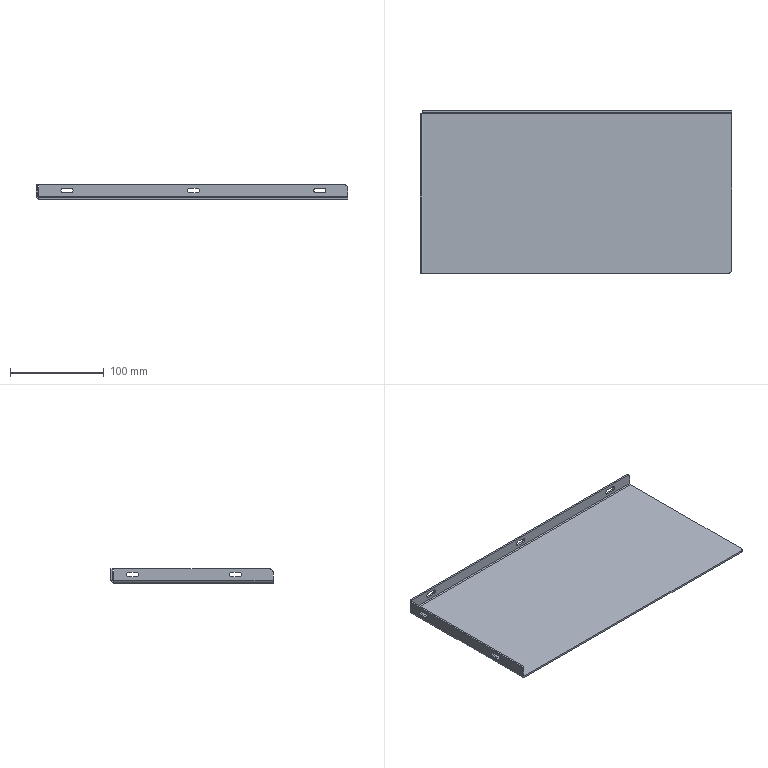Part | NX | features BREP 1 | 1 solid | 45 faces | box 333 x 173 x 15 mm | volume 126734 mm3 | plane 28 | cylinder 17 | commonest cylinder face diameters 5 x10 6 x5 2 x2
STEP:
#1=CARTESIAN_POINT('',(-168.,-85.,10.));
#2=VERTEX_POINT('',#1);
#3=CARTESIAN_POINT('',(-168.,-82.,13.));
#4=VERTEX_POINT('',#3);
#5=CARTESIAN_POINT('',(-168.,-82.,10.));
#6=DIRECTION('',(-1.,0.,0.));
#7=DIRECTION('',(0.,0.,-1.));
#8=AXIS2_PLACEMENT_3D('',#5,#6,#7);
#9=CIRCLE('',#8,3.);
#10=EDGE_CURVE('',#2,#4,#9,.T.);
#11=ORIENTED_EDGE('',*,*,#10,.F.);
#12=CARTESIAN_POINT('',(-166.,-85.,10.));
#13=VERTEX_POINT('',#12);
#14=CARTESIAN_POINT('',(-168.,-85.,10.));
#15=DIRECTION('',(-1.,0.,0.));
#16=VECTOR('',#15,1000.);
#17=LINE('',#14,#16);
#18=EDGE_CURVE('',#13,#2,#17,.T.);
#19=ORIENTED_EDGE('',*,*,#18,.F.);
#20=CARTESIAN_POINT('',(-166.,-82.,13.));
#21=VERTEX_POINT('',#20);
#22=CARTESIAN_POINT('',(-166.,-82.,10.));
#23=DIRECTION('',(1.,0.,0.));
#24=DIRECTION('',(0.,0.,-1.));
#25=AXIS2_PLACEMENT_3D('',#22,#23,#24);
#26=CIRCLE('',#25,3.);
#27=EDGE_CURVE('',#21,#13,#26,.T.);
#28=ORIENTED_EDGE('',*,*,#27,.F.);
#29=CARTESIAN_POINT('',(-168.,-82.,13.));
#30=DIRECTION('',(1.,0.,0.));
#31=VECTOR('',#30,1000.);
#32=LINE('',#29,#31);
#33=EDGE_CURVE('',#4,#21,#32,.T.);
#34=ORIENTED_EDGE('',*,*,#33,.F.);
#35=EDGE_LOOP('',(#11,#19,#28,#34));
#36=FACE_BOUND('',#35,.T.);
#37=CARTESIAN_POINT('',(-168.,-82.,10.));
#38=DIRECTION('',(1.,0.,0.));
#39=DIRECTION('',(0.,0.,-1.));
#40=AXIS2_PLACEMENT_3D('',#37,#38,#39);
#41=CYLINDRICAL_SURFACE('',#40,3.);
#42=ADVANCED_FACE('',(#36),#41,.T.);
#43=CARTESIAN_POINT('',(165.,-82.,-2.));
#44=VERTEX_POINT('',#43);
#45=CARTESIAN_POINT('',(162.,-85.,-2.));
#46=VERTEX_POINT('',#45);
#47=CARTESIAN_POINT('',(162.,-82.,-2.));
#48=DIRECTION('',(0.,0.,-1.));
#49=DIRECTION('',(-1.,0.,0.));
#50=AXIS2_PLACEMENT_3D('',#47,#48,#49);
#51=CIRCLE('',#50,3.);
#52=EDGE_CURVE('',#44,#46,#51,.T.);
#53=ORIENTED_EDGE('',*,*,#52,.F.);
#54=CARTESIAN_POINT('',(165.,-82.,0.));
#55=VERTEX_POINT('',#54);
#56=CARTESIAN_POINT('',(165.,-82.,-2.));
#57=DIRECTION('',(0.,0.,-1.));
#58=VECTOR('',#57,1000.);
#59=LINE('',#56,#58);
#60=EDGE_CURVE('',#55,#44,#59,.T.);
#61=ORIENTED_EDGE('',*,*,#60,.F.);
#62=CARTESIAN_POINT('',(162.,-85.,0.));
#63=VERTEX_POINT('',#62);
#64=CARTESIAN_POINT('',(162.,-82.,0.));
#65=DIRECTION('',(0.,0.,1.));
#66=DIRECTION('',(-1.,0.,0.));
#67=AXIS2_PLACEMENT_3D('',#64,#65,#66);
#68=CIRCLE('',#67,3.);
#69=EDGE_CURVE('',#63,#55,#68,.T.);
#70=ORIENTED_EDGE('',*,*,#69,.F.);
#71=CARTESIAN_POINT('',(162.,-85.,-2.));
#72=DIRECTION('',(0.,0.,1.));
#73=VECTOR('',#72,1000.);
#74=LINE('',#71,#73);
#75=EDGE_CURVE('',#46,#63,#74,.T.);
#76=ORIENTED_EDGE('',*,*,#75,.F.);
#77=EDGE_LOOP('',(#53,#61,#70,#76));
#78=FACE_BOUND('',#77,.T.);
#79=CARTESIAN_POINT('',(162.,-82.,-2.));
#80=DIRECTION('',(0.,0.,1.));
#81=DIRECTION('',(1.,0.,0.));
#82=AXIS2_PLACEMENT_3D('',#79,#80,#81);
#83=CYLINDRICAL_SURFACE('',#82,3.);
#84=ADVANCED_FACE('',(#78),#83,.T.);
#85=CARTESIAN_POINT('',(162.,88.,13.));
#86=VERTEX_POINT('',#85);
#87=CARTESIAN_POINT('',(165.,88.,10.));
#88=VERTEX_POINT('',#87);
#89=CARTESIAN_POINT('',(162.,88.,10.));
#90=DIRECTION('',(0.,1.,0.));
#91=DIRECTION('',(0.,0.,-1.));
#92=AXIS2_PLACEMENT_3D('',#89,#90,#91);
#93=CIRCLE('',#92,3.);
#94=EDGE_CURVE('',#86,#88,#93,.T.);
#95=ORIENTED_EDGE('',*,*,#94,.F.);
#96=CARTESIAN_POINT('',(162.,86.,13.));
#97=VERTEX_POINT('',#96);
#98=CARTESIAN_POINT('',(162.,88.,13.));
#99=DIRECTION('',(0.,1.,0.));
#100=VECTOR('',#99,1000.);
#101=LINE('',#98,#100);
#102=EDGE_CURVE('',#97,#86,#101,.T.);
#103=ORIENTED_EDGE('',*,*,#102,.F.);
#104=CARTESIAN_POINT('',(165.,86.,10.));
#105=VERTEX_POINT('',#104);
#106=CARTESIAN_POINT('',(162.,86.,10.));
#107=DIRECTION('',(0.,-1.,0.));
#108=DIRECTION('',(0.,0.,-1.));
#109=AXIS2_PLACEMENT_3D('',#106,#107,#108);
#110=CIRCLE('',#109,3.);
#111=EDGE_CURVE('',#105,#97,#110,.T.);
#112=ORIENTED_EDGE('',*,*,#111,.F.);
#113=CARTESIAN_POINT('',(165.,88.,10.));
#114=DIRECTION('',(0.,-1.,0.));
#115=VECTOR('',#114,1000.);
#116=LINE('',#113,#115);
#117=EDGE_CURVE('',#88,#105,#116,.T.);
#118=ORIENTED_EDGE('',*,*,#117,.F.);
#119=EDGE_LOOP('',(#95,#103,#112,#118));
#120=FACE_BOUND('',#119,.T.);
#121=CARTESIAN_POINT('',(162.,88.,10.));
#122=DIRECTION('',(0.,-1.,0.));
#123=DIRECTION('',(0.,0.,-1.));
#124=AXIS2_PLACEMENT_3D('',#121,#122,#123);
#125=CYLINDRICAL_SURFACE('',#124,3.);
#126=ADVANCED_FACE('',(#120),#125,.T.);
#127=CARTESIAN_POINT('',(-166.,-49.,4.5));
#128=VERTEX_POINT('',#127);
#129=CARTESIAN_POINT('',(-166.,-41.,4.5));
#130=VERTEX_POINT('',#129);
#131=CARTESIAN_POINT('',(-166.,-49.,4.5));
#132=DIRECTION('',(0.,1.,0.));
#133=VECTOR('',#132,1000.);
#134=LINE('',#131,#133);
#135=EDGE_CURVE('',#128,#130,#134,.T.);
#136=ORIENTED_EDGE('',*,*,#135,.T.);
#137=CARTESIAN_POINT('',(-168.,-41.,4.5));
#138=VERTEX_POINT('',#137);
#139=CARTESIAN_POINT('',(-168.,-41.,4.5));
#140=DIRECTION('',(1.,0.,0.));
#141=VECTOR('',#140,1000.);
#142=LINE('',#139,#141);
#143=EDGE_CURVE('',#138,#130,#142,.T.);
#144=ORIENTED_EDGE('',*,*,#143,.F.);
#145=CARTESIAN_POINT('',(-168.,-49.,4.5));
#146=VERTEX_POINT('',#145);
#147=CARTESIAN_POINT('',(-168.,-49.,4.5));
#148=DIRECTION('',(0.,1.,0.));
#149=VECTOR('',#148,1000.);
#150=LINE('',#147,#149);
#151=EDGE_CURVE('',#146,#138,#150,.T.);
#152=ORIENTED_EDGE('',*,*,#151,.F.);
#153=CARTESIAN_POINT('',(-168.,-49.,4.5));
#154=DIRECTION('',(1.,0.,0.));
#155=VECTOR('',#154,1000.);
#156=LINE('',#153,#155);
#157=EDGE_CURVE('',#146,#128,#156,.T.);
#158=ORIENTED_EDGE('',*,*,#157,.T.);
#159=EDGE_LOOP('',(#136,#144,#152,#158));
#160=FACE_BOUND('',#159,.T.);
#161=CARTESIAN_POINT('',(-168.,-49.,4.5));
#162=DIRECTION('',(0.,0.,-1.));
#163=DIRECTION('',(-1.,0.,0.));
#164=AXIS2_PLACEMENT_3D('',#161,#162,#163);
#165=PLANE('',#164);
#166=ADVANCED_FACE('',(#160),#165,.F.);
#167=CARTESIAN_POINT('',(-166.,-41.,9.5));
#168=VERTEX_POINT('',#167);
#169=CARTESIAN_POINT('',(-166.,-41.,7.));
#170=DIRECTION('',(1.,0.,0.));
#171=DIRECTION('',(0.,0.,-1.));
#172=AXIS2_PLACEMENT_3D('',#169,#170,#171);
#173=CIRCLE('',#172,2.5);
#174=EDGE_CURVE('',#130,#168,#173,.T.);
#175=ORIENTED_EDGE('',*,*,#174,.T.);
#176=CARTESIAN_POINT('',(-168.,-41.,9.5));
#177=VERTEX_POINT('',#176);
#178=CARTESIAN_POINT('',(-168.,-41.,9.5));
#179=DIRECTION('',(1.,0.,0.));
#180=VECTOR('',#179,1000.);
#181=LINE('',#178,#180);
#182=EDGE_CURVE('',#177,#168,#181,.T.);
#183=ORIENTED_EDGE('',*,*,#182,.F.);
#184=CARTESIAN_POINT('',(-168.,-41.,7.));
#185=DIRECTION('',(1.,0.,0.));
#186=DIRECTION('',(0.,0.,-1.));
#187=AXIS2_PLACEMENT_3D('',#184,#185,#186);
#188=CIRCLE('',#187,2.5);
#189=EDGE_CURVE('',#138,#177,#188,.T.);
#190=ORIENTED_EDGE('',*,*,#189,.F.);
#191=ORIENTED_EDGE('',*,*,#143,.T.);
#192=EDGE_LOOP('',(#175,#183,#190,#191));
#193=FACE_BOUND('',#192,.T.);
#194=CARTESIAN_POINT('',(-168.,-41.,7.));
#195=DIRECTION('',(1.,0.,0.));
#196=DIRECTION('',(0.,0.,-1.));
#197=AXIS2_PLACEMENT_3D('',#194,#195,#196);
#198=CYLINDRICAL_SURFACE('',#197,2.5);
#199=ADVANCED_FACE('',(#193),#198,.F.);
#200=CARTESIAN_POINT('',(-166.,-49.,9.5));
#201=VERTEX_POINT('',#200);
#202=CARTESIAN_POINT('',(-166.,-49.,9.5));
#203=DIRECTION('',(0.,-1.,0.));
#204=VECTOR('',#203,1000.);
#205=LINE('',#202,#204);
#206=EDGE_CURVE('',#168,#201,#205,.T.);
#207=ORIENTED_EDGE('',*,*,#206,.T.);
#208=CARTESIAN_POINT('',(-168.,-49.,9.5));
#209=VERTEX_POINT('',#208);
#210=CARTESIAN_POINT('',(-168.,-49.,9.5));
#211=DIRECTION('',(1.,0.,0.));
#212=VECTOR('',#211,1000.);
#213=LINE('',#210,#212);
#214=EDGE_CURVE('',#209,#201,#213,.T.);
#215=ORIENTED_EDGE('',*,*,#214,.F.);
#216=CARTESIAN_POINT('',(-168.,-49.,9.5));
#217=DIRECTION('',(0.,-1.,0.));
#218=VECTOR('',#217,1000.);
#219=LINE('',#216,#218);
#220=EDGE_CURVE('',#177,#209,#219,.T.);
#221=ORIENTED_EDGE('',*,*,#220,.F.);
#222=ORIENTED_EDGE('',*,*,#182,.T.);
#223=EDGE_LOOP('',(#207,#215,#221,#222));
#224=FACE_BOUND('',#223,.T.);
#225=CARTESIAN_POINT('',(-168.,-49.,9.5));
#226=DIRECTION('',(0.,0.,1.));
#227=DIRECTION('',(1.,0.,0.));
#228=AXIS2_PLACEMENT_3D('',#225,#226,#227);
#229=PLANE('',#228);
#230=ADVANCED_FACE('',(#224),#229,.F.);
#231=CARTESIAN_POINT('',(-166.,-49.,7.));
#232=DIRECTION('',(1.,0.,0.));
#233=DIRECTION('',(0.,0.,-1.));
#234=AXIS2_PLACEMENT_3D('',#231,#232,#233);
#235=CIRCLE('',#234,2.5);
#236=EDGE_CURVE('',#201,#128,#235,.T.);
#237=ORIENTED_EDGE('',*,*,#236,.T.);
#238=ORIENTED_EDGE('',*,*,#157,.F.);
#239=CARTESIAN_POINT('',(-168.,-49.,7.));
#240=DIRECTION('',(1.,0.,0.));
#241=DIRECTION('',(0.,0.,-1.));
#242=AXIS2_PLACEMENT_3D('',#239,#240,#241);
#243=CIRCLE('',#242,2.5);
#244=EDGE_CURVE('',#209,#146,#243,.T.);
#245=ORIENTED_EDGE('',*,*,#244,.F.);
#246=ORIENTED_EDGE('',*,*,#214,.T.);
#247=EDGE_LOOP('',(#237,#238,#245,#246));
#248=FACE_BOUND('',#247,.T.);
#249=CARTESIAN_POINT('',(-168.,-49.,7.));
#250=DIRECTION('',(1.,0.,0.));
#251=DIRECTION('',(0.,0.,-1.));
#252=AXIS2_PLACEMENT_3D('',#249,#250,#251);
#253=CYLINDRICAL_SURFACE('',#252,2.5);
#254=ADVANCED_FACE('',(#248),#253,.F.);
#255=CARTESIAN_POINT('',(-166.,61.,4.5));
#256=VERTEX_POINT('',#255);
#257=CARTESIAN_POINT('',(-166.,69.,4.5));
#258=VERTEX_POINT('',#257);
#259=CARTESIAN_POINT('',(-166.,61.,4.5));
#260=DIRECTION('',(0.,1.,0.));
#261=VECTOR('',#260,1000.);
#262=LINE('',#259,#261);
#263=EDGE_CURVE('',#256,#258,#262,.T.);
#264=ORIENTED_EDGE('',*,*,#263,.T.);
#265=CARTESIAN_POINT('',(-168.,69.,4.5));
#266=VERTEX_POINT('',#265);
#267=CARTESIAN_POINT('',(-168.,69.,4.5));
#268=DIRECTION('',(1.,0.,0.));
#269=VECTOR('',#268,1000.);
#270=LINE('',#267,#269);
#271=EDGE_CURVE('',#266,#258,#270,.T.);
#272=ORIENTED_EDGE('',*,*,#271,.F.);
#273=CARTESIAN_POINT('',(-168.,61.,4.5));
#274=VERTEX_POINT('',#273);
#275=CARTESIAN_POINT('',(-168.,61.,4.5));
#276=DIRECTION('',(0.,1.,0.));
#277=VECTOR('',#276,1000.);
#278=LINE('',#275,#277);
#279=EDGE_CURVE('',#274,#266,#278,.T.);
#280=ORIENTED_EDGE('',*,*,#279,.F.);
#281=CARTESIAN_POINT('',(-168.,61.,4.5));
#282=DIRECTION('',(1.,0.,0.));
#283=VECTOR('',#282,1000.);
#284=LINE('',#281,#283);
#285=EDGE_CURVE('',#274,#256,#284,.T.);
#286=ORIENTED_EDGE('',*,*,#285,.T.);
#287=EDGE_LOOP('',(#264,#272,#280,#286));
#288=FACE_BOUND('',#287,.T.);
#289=CARTESIAN_POINT('',(-168.,61.,4.5));
#290=DIRECTION('',(0.,0.,-1.));
#291=DIRECTION('',(-1.,0.,0.));
#292=AXIS2_PLACEMENT_3D('',#289,#290,#291);
#293=PLANE('',#292);
#294=ADVANCED_FACE('',(#288),#293,.F.);
#295=CARTESIAN_POINT('',(-166.,69.,9.5));
#296=VERTEX_POINT('',#295);
#297=CARTESIAN_POINT('',(-166.,69.,7.));
#298=DIRECTION('',(1.,0.,0.));
#299=DIRECTION('',(0.,0.,-1.));
#300=AXIS2_PLACEMENT_3D('',#297,#298,#299);
#301=CIRCLE('',#300,2.5);
#302=EDGE_CURVE('',#258,#296,#301,.T.);
#303=ORIENTED_EDGE('',*,*,#302,.T.);
#304=CARTESIAN_POINT('',(-168.,69.,9.5));
#305=VERTEX_POINT('',#304);
#306=CARTESIAN_POINT('',(-168.,69.,9.5));
#307=DIRECTION('',(1.,0.,0.));
#308=VECTOR('',#307,1000.);
#309=LINE('',#306,#308);
#310=EDGE_CURVE('',#305,#296,#309,.T.);
#311=ORIENTED_EDGE('',*,*,#310,.F.);
#312=CARTESIAN_POINT('',(-168.,69.,7.));
#313=DIRECTION('',(1.,0.,0.));
#314=DIRECTION('',(0.,0.,-1.));
#315=AXIS2_PLACEMENT_3D('',#312,#313,#314);
#316=CIRCLE('',#315,2.5);
#317=EDGE_CURVE('',#266,#305,#316,.T.);
#318=ORIENTED_EDGE('',*,*,#317,.F.);
#319=ORIENTED_EDGE('',*,*,#271,.T.);
#320=EDGE_LOOP('',(#303,#311,#318,#319));
#321=FACE_BOUND('',#320,.T.);
#322=CARTESIAN_POINT('',(-168.,69.,7.));
#323=DIRECTION('',(1.,0.,0.));
#324=DIRECTION('',(0.,0.,-1.));
#325=AXIS2_PLACEMENT_3D('',#322,#323,#324);
#326=CYLINDRICAL_SURFACE('',#325,2.5);
#327=ADVANCED_FACE('',(#321),#326,.F.);
#328=CARTESIAN_POINT('',(-166.,61.,9.5));
#329=VERTEX_POINT('',#328);
#330=CARTESIAN_POINT('',(-166.,61.,9.5));
#331=DIRECTION('',(0.,-1.,0.));
#332=VECTOR('',#331,1000.);
#333=LINE('',#330,#332);
#334=EDGE_CURVE('',#296,#329,#333,.T.);
#335=ORIENTED_EDGE('',*,*,#334,.T.);
#336=CARTESIAN_POINT('',(-168.,61.,9.5));
#337=VERTEX_POINT('',#336);
#338=CARTESIAN_POINT('',(-168.,61.,9.5));
#339=DIRECTION('',(1.,0.,0.));
#340=VECTOR('',#339,1000.);
#341=LINE('',#338,#340);
#342=EDGE_CURVE('',#337,#329,#341,.T.);
#343=ORIENTED_EDGE('',*,*,#342,.F.);
#344=CARTESIAN_POINT('',(-168.,61.,9.5));
#345=DIRECTION('',(0.,-1.,0.));
#346=VECTOR('',#345,1000.);
#347=LINE('',#344,#346);
#348=EDGE_CURVE('',#305,#337,#347,.T.);
#349=ORIENTED_EDGE('',*,*,#348,.F.);
#350=ORIENTED_EDGE('',*,*,#310,.T.);
#351=EDGE_LOOP('',(#335,#343,#349,#350));
#352=FACE_BOUND('',#351,.T.);
#353=CARTESIAN_POINT('',(-168.,61.,9.5));
#354=DIRECTION('',(0.,0.,1.));
#355=DIRECTION('',(1.,0.,0.));
#356=AXIS2_PLACEMENT_3D('',#353,#354,#355);
#357=PLANE('',#356);
#358=ADVANCED_FACE('',(#352),#357,.F.);
#359=CARTESIAN_POINT('',(-166.,61.,7.));
#360=DIRECTION('',(1.,0.,0.));
#361=DIRECTION('',(0.,0.,-1.));
#362=AXIS2_PLACEMENT_3D('',#359,#360,#361);
#363=CIRCLE('',#362,2.5);
#364=EDGE_CURVE('',#329,#256,#363,.T.);
#365=ORIENTED_EDGE('',*,*,#364,.T.);
#366=ORIENTED_EDGE('',*,*,#285,.F.);
#367=CARTESIAN_POINT('',(-168.,61.,7.));
#368=DIRECTION('',(1.,0.,0.));
#369=DIRECTION('',(0.,0.,-1.));
#370=AXIS2_PLACEMENT_3D('',#367,#368,#369);
#371=CIRCLE('',#370,2.5);
#372=EDGE_CURVE('',#337,#274,#371,.T.);
#373=ORIENTED_EDGE('',*,*,#372,.F.);
#374=ORIENTED_EDGE('',*,*,#342,.T.);
#375=EDGE_LOOP('',(#365,#366,#373,#374));
#376=FACE_BOUND('',#375,.T.);
#377=CARTESIAN_POINT('',(-168.,61.,7.));
#378=DIRECTION('',(1.,0.,0.));
#379=DIRECTION('',(0.,0.,-1.));
#380=AXIS2_PLACEMENT_3D('',#377,#378,#379);
#381=CYLINDRICAL_SURFACE('',#380,2.5);
#382=ADVANCED_FACE('',(#376),#381,.F.);
#383=CARTESIAN_POINT('',(4.,86.,9.5));
#384=VERTEX_POINT('',#383);
#385=CARTESIAN_POINT('',(-4.,86.,9.5));
#386=VERTEX_POINT('',#385);
#387=CARTESIAN_POINT('',(4.,86.,9.5));
#388=DIRECTION('',(-1.,0.,0.));
#389=VECTOR('',#388,1000.);
#390=LINE('',#387,#389);
#391=EDGE_CURVE('',#384,#386,#390,.T.);
#392=ORIENTED_EDGE('',*,*,#391,.T.);
#393=CARTESIAN_POINT('',(-4.,88.,9.5));
#394=VERTEX_POINT('',#393);
#395=CARTESIAN_POINT('',(-4.,88.,9.5));
#396=DIRECTION('',(0.,-1.,0.));
#397=VECTOR('',#396,1000.);
#398=LINE('',#395,#397);
#399=EDGE_CURVE('',#394,#386,#398,.T.);
#400=ORIENTED_EDGE('',*,*,#399,.F.);
#401=CARTESIAN_POINT('',(4.,88.,9.5));
#402=VERTEX_POINT('',#401);
#403=CARTESIAN_POINT('',(4.,88.,9.5));
#404=DIRECTION('',(-1.,0.,0.));
#405=VECTOR('',#404,1000.);
#406=LINE('',#403,#405);
#407=EDGE_CURVE('',#402,#394,#406,.T.);
#408=ORIENTED_EDGE('',*,*,#407,.F.);
#409=CARTESIAN_POINT('',(4.,88.,9.5));
#410=DIRECTION('',(0.,-1.,0.));
#411=VECTOR('',#410,1000.);
#412=LINE('',#409,#411);
#413=EDGE_CURVE('',#402,#384,#412,.T.);
#414=ORIENTED_EDGE('',*,*,#413,.T.);
#415=EDGE_LOOP('',(#392,#400,#408,#414));
#416=FACE_BOUND('',#415,.T.);
#417=CARTESIAN_POINT('',(4.,88.,9.5));
#418=DIRECTION('',(0.,0.,1.));
#419=DIRECTION('',(0.,-1.,0.));
#420=AXIS2_PLACEMENT_3D('',#417,#418,#419);
#421=PLANE('',#420);
#422=ADVANCED_FACE('',(#416),#421,.F.);
#423=CARTESIAN_POINT('',(-4.,86.,4.5));
#424=VERTEX_POINT('',#423);
#425=CARTESIAN_POINT('',(-4.,86.,7.));
#426=DIRECTION('',(0.,-1.,0.));
#427=DIRECTION('',(0.,0.,-1.));
#428=AXIS2_PLACEMENT_3D('',#425,#426,#427);
#429=CIRCLE('',#428,2.5);
#430=EDGE_CURVE('',#386,#424,#429,.T.);
#431=ORIENTED_EDGE('',*,*,#430,.T.);
#432=CARTESIAN_POINT('',(-4.,88.,4.5));
#433=VERTEX_POINT('',#432);
#434=CARTESIAN_POINT('',(-4.,88.,4.5));
#435=DIRECTION('',(0.,-1.,0.));
#436=VECTOR('',#435,1000.);
#437=LINE('',#434,#436);
#438=EDGE_CURVE('',#433,#424,#437,.T.);
#439=ORIENTED_EDGE('',*,*,#438,.F.);
#440=CARTESIAN_POINT('',(-4.,88.,7.));
#441=DIRECTION('',(0.,-1.,0.));
#442=DIRECTION('',(0.,0.,-1.));
#443=AXIS2_PLACEMENT_3D('',#440,#441,#442);
#444=CIRCLE('',#443,2.5);
#445=EDGE_CURVE('',#394,#433,#444,.T.);
#446=ORIENTED_EDGE('',*,*,#445,.F.);
#447=ORIENTED_EDGE('',*,*,#399,.T.);
#448=EDGE_LOOP('',(#431,#439,#446,#447));
#449=FACE_BOUND('',#448,.T.);
#450=CARTESIAN_POINT('',(-4.,88.,7.));
#451=DIRECTION('',(0.,-1.,0.));
#452=DIRECTION('',(0.,0.,-1.));
#453=AXIS2_PLACEMENT_3D('',#450,#451,#452);
#454=CYLINDRICAL_SURFACE('',#453,2.5);
#455=ADVANCED_FACE('',(#449),#454,.F.);
#456=CARTESIAN_POINT('',(4.,86.,4.5));
#457=VERTEX_POINT('',#456);
#458=CARTESIAN_POINT('',(4.,86.,4.5));
#459=DIRECTION('',(1.,0.,0.));
#460=VECTOR('',#459,1000.);
#461=LINE('',#458,#460);
#462=EDGE_CURVE('',#424,#457,#461,.T.);
#463=ORIENTED_EDGE('',*,*,#462,.T.);
#464=CARTESIAN_POINT('',(4.,88.,4.5));
#465=VERTEX_POINT('',#464);
#466=CARTESIAN_POINT('',(4.,88.,4.5));
#467=DIRECTION('',(0.,-1.,0.));
#468=VECTOR('',#467,1000.);
#469=LINE('',#466,#468);
#470=EDGE_CURVE('',#465,#457,#469,.T.);
#471=ORIENTED_EDGE('',*,*,#470,.F.);
#472=CARTESIAN_POINT('',(4.,88.,4.5));
#473=DIRECTION('',(1.,0.,0.));
#474=VECTOR('',#473,1000.);
#475=LINE('',#472,#474);
#476=EDGE_CURVE('',#433,#465,#475,.T.);
#477=ORIENTED_EDGE('',*,*,#476,.F.);
#478=ORIENTED_EDGE('',*,*,#438,.T.);
#479=EDGE_LOOP('',(#463,#471,#477,#478));
#480=FACE_BOUND('',#479,.T.);
#481=CARTESIAN_POINT('',(4.,88.,4.5));
#482=DIRECTION('',(0.,0.,-1.));
#483=DIRECTION('',(0.,1.,0.));
#484=AXIS2_PLACEMENT_3D('',#481,#482,#483);
#485=PLANE('',#484);
#486=ADVANCED_FACE('',(#480),#485,.F.);
#487=CARTESIAN_POINT('',(4.,86.,7.));
#488=DIRECTION('',(0.,-1.,0.));
#489=DIRECTION('',(0.,0.,-1.));
#490=AXIS2_PLACEMENT_3D('',#487,#488,#489);
#491=CIRCLE('',#490,2.5);
#492=EDGE_CURVE('',#457,#384,#491,.T.);
#493=ORIENTED_EDGE('',*,*,#492,.T.);
#494=ORIENTED_EDGE('',*,*,#413,.F.);
#495=CARTESIAN_POINT('',(4.,88.,7.));
#496=DIRECTION('',(0.,-1.,0.));
#497=DIRECTION('',(0.,0.,-1.));
#498=AXIS2_PLACEMENT_3D('',#495,#496,#497);
#499=CIRCLE('',#498,2.5);
#500=EDGE_CURVE('',#465,#402,#499,.T.);
#501=ORIENTED_EDGE('',*,*,#500,.F.);
#502=ORIENTED_EDGE('',*,*,#470,.T.);
#503=EDGE_LOOP('',(#493,#494,#501,#502));
#504=FACE_BOUND('',#503,.T.);
#505=CARTESIAN_POINT('',(4.,88.,7.));
#506=DIRECTION('',(0.,-1.,0.));
#507=DIRECTION('',(0.,0.,-1.));
#508=AXIS2_PLACEMENT_3D('',#505,#506,#507);
#509=CYLINDRICAL_SURFACE('',#508,2.5);
#510=ADVANCED_FACE('',(#504),#509,.F.);
#511=CARTESIAN_POINT('',(-131.,86.,9.5));
#512=VERTEX_POINT('',#511);
#513=CARTESIAN_POINT('',(-139.,86.,9.5));
#514=VERTEX_POINT('',#513);
#515=CARTESIAN_POINT('',(-131.,86.,9.5));
#516=DIRECTION('',(-1.,0.,0.));
#517=VECTOR('',#516,1000.);
#518=LINE('',#515,#517);
#519=EDGE_CURVE('',#512,#514,#518,.T.);
#520=ORIENTED_EDGE('',*,*,#519,.T.);
#521=CARTESIAN_POINT('',(-139.,88.,9.5));
#522=VERTEX_POINT('',#521);
#523=CARTESIAN_POINT('',(-139.,88.,9.5));
#524=DIRECTION('',(0.,-1.,0.));
#525=VECTOR('',#524,1000.);
#526=LINE('',#523,#525);
#527=EDGE_CURVE('',#522,#514,#526,.T.);
#528=ORIENTED_EDGE('',*,*,#527,.F.);
#529=CARTESIAN_POINT('',(-131.,88.,9.5));
#530=VERTEX_POINT('',#529);
#531=CARTESIAN_POINT('',(-131.,88.,9.5));
#532=DIRECTION('',(-1.,0.,0.));
#533=VECTOR('',#532,1000.);
#534=LINE('',#531,#533);
#535=EDGE_CURVE('',#530,#522,#534,.T.);
#536=ORIENTED_EDGE('',*,*,#535,.F.);
#537=CARTESIAN_POINT('',(-131.,88.,9.5));
#538=DIRECTION('',(0.,-1.,0.));
#539=VECTOR('',#538,1000.);
#540=LINE('',#537,#539);
#541=EDGE_CURVE('',#530,#512,#540,.T.);
#542=ORIENTED_EDGE('',*,*,#541,.T.);
#543=EDGE_LOOP('',(#520,#528,#536,#542));
#544=FACE_BOUND('',#543,.T.);
#545=CARTESIAN_POINT('',(-131.,88.,9.5));
#546=DIRECTION('',(0.,0.,1.));
#547=DIRECTION('',(0.,-1.,0.));
#548=AXIS2_PLACEMENT_3D('',#545,#546,#547);
#549=PLANE('',#548);
#550=ADVANCED_FACE('',(#544),#549,.F.);
#551=CARTESIAN_POINT('',(-139.,86.,4.5));
#552=VERTEX_POINT('',#551);
#553=CARTESIAN_POINT('',(-139.,86.,7.));
#554=DIRECTION('',(0.,-1.,0.));
#555=DIRECTION('',(0.,0.,-1.));
#556=AXIS2_PLACEMENT_3D('',#553,#554,#555);
#557=CIRCLE('',#556,2.5);
#558=EDGE_CURVE('',#514,#552,#557,.T.);
#559=ORIENTED_EDGE('',*,*,#558,.T.);
#560=CARTESIAN_POINT('',(-139.,88.,4.5));
#561=VERTEX_POINT('',#560);
#562=CARTESIAN_POINT('',(-139.,88.,4.5));
#563=DIRECTION('',(0.,-1.,0.));
#564=VECTOR('',#563,1000.);
#565=LINE('',#562,#564);
#566=EDGE_CURVE('',#561,#552,#565,.T.);
#567=ORIENTED_EDGE('',*,*,#566,.F.);
#568=CARTESIAN_POINT('',(-139.,88.,7.));
#569=DIRECTION('',(0.,-1.,0.));
#570=DIRECTION('',(0.,0.,-1.));
#571=AXIS2_PLACEMENT_3D('',#568,#569,#570);
#572=CIRCLE('',#571,2.5);
#573=EDGE_CURVE('',#522,#561,#572,.T.);
#574=ORIENTED_EDGE('',*,*,#573,.F.);
#575=ORIENTED_EDGE('',*,*,#527,.T.);
#576=EDGE_LOOP('',(#559,#567,#574,#575));
#577=FACE_BOUND('',#576,.T.);
#578=CARTESIAN_POINT('',(-139.,88.,7.));
#579=DIRECTION('',(0.,-1.,0.));
#580=DIRECTION('',(0.,0.,-1.));
#581=AXIS2_PLACEMENT_3D('',#578,#579,#580);
#582=CYLINDRICAL_SURFACE('',#581,2.5);
#583=ADVANCED_FACE('',(#577),#582,.F.);
#584=CARTESIAN_POINT('',(-131.,86.,4.5));
#585=VERTEX_POINT('',#584);
#586=CARTESIAN_POINT('',(-131.,86.,4.5));
#587=DIRECTION('',(1.,0.,0.));
#588=VECTOR('',#587,1000.);
#589=LINE('',#586,#588);
#590=EDGE_CURVE('',#552,#585,#589,.T.);
#591=ORIENTED_EDGE('',*,*,#590,.T.);
#592=CARTESIAN_POINT('',(-131.,88.,4.5));
#593=VERTEX_POINT('',#592);
#594=CARTESIAN_POINT('',(-131.,88.,4.5));
#595=DIRECTION('',(0.,-1.,0.));
#596=VECTOR('',#595,1000.);
#597=LINE('',#594,#596);
#598=EDGE_CURVE('',#593,#585,#597,.T.);
#599=ORIENTED_EDGE('',*,*,#598,.F.);
#600=CARTESIAN_POINT('',(-131.,88.,4.5));
#601=DIRECTION('',(1.,0.,0.));
#602=VECTOR('',#601,1000.);
#603=LINE('',#600,#602);
#604=EDGE_CURVE('',#561,#593,#603,.T.);
#605=ORIENTED_EDGE('',*,*,#604,.F.);
#606=ORIENTED_EDGE('',*,*,#566,.T.);
#607=EDGE_LOOP('',(#591,#599,#605,#606));
#608=FACE_BOUND('',#607,.T.);
#609=CARTESIAN_POINT('',(-131.,88.,4.5));
#610=DIRECTION('',(0.,0.,-1.));
#611=DIRECTION('',(0.,1.,0.));
#612=AXIS2_PLACEMENT_3D('',#609,#610,#611);
#613=PLANE('',#612);
#614=ADVANCED_FACE('',(#608),#613,.F.);
#615=CARTESIAN_POINT('',(-131.,86.,7.));
#616=DIRECTION('',(0.,-1.,0.));
#617=DIRECTION('',(0.,0.,-1.));
#618=AXIS2_PLACEMENT_3D('',#615,#616,#617);
#619=CIRCLE('',#618,2.5);
#620=EDGE_CURVE('',#585,#512,#619,.T.);
#621=ORIENTED_EDGE('',*,*,#620,.T.);
#622=ORIENTED_EDGE('',*,*,#541,.F.);
#623=CARTESIAN_POINT('',(-131.,88.,7.));
#624=DIRECTION('',(0.,-1.,0.));
#625=DIRECTION('',(0.,0.,-1.));
#626=AXIS2_PLACEMENT_3D('',#623,#624,#625);
#627=CIRCLE('',#626,2.5);
#628=EDGE_CURVE('',#593,#530,#627,.T.);
#629=ORIENTED_EDGE('',*,*,#628,.F.);
#630=ORIENTED_EDGE('',*,*,#598,.T.);
#631=EDGE_LOOP('',(#621,#622,#629,#630));
#632=FACE_BOUND('',#631,.T.);
#633=CARTESIAN_POINT('',(-131.,88.,7.));
#634=DIRECTION('',(0.,-1.,0.));
#635=DIRECTION('',(0.,0.,-1.));
#636=AXIS2_PLACEMENT_3D('',#633,#634,#635);
#637=CYLINDRICAL_SURFACE('',#636,2.5);
#638=ADVANCED_FACE('',(#632),#637,.F.);
#639=CARTESIAN_POINT('',(139.,86.,9.5));
#640=VERTEX_POINT('',#639);
#641=CARTESIAN_POINT('',(131.,86.,9.5));
#642=VERTEX_POINT('',#641);
#643=CARTESIAN_POINT('',(139.,86.,9.5));
#644=DIRECTION('',(-1.,0.,0.));
#645=VECTOR('',#644,1000.);
#646=LINE('',#643,#645);
#647=EDGE_CURVE('',#640,#642,#646,.T.);
#648=ORIENTED_EDGE('',*,*,#647,.T.);
#649=CARTESIAN_POINT('',(131.,88.,9.5));
#650=VERTEX_POINT('',#649);
#651=CARTESIAN_POINT('',(131.,88.,9.5));
#652=DIRECTION('',(0.,-1.,0.));
#653=VECTOR('',#652,1000.);
#654=LINE('',#651,#653);
#655=EDGE_CURVE('',#650,#642,#654,.T.);
#656=ORIENTED_EDGE('',*,*,#655,.F.);
#657=CARTESIAN_POINT('',(139.,88.,9.5));
#658=VERTEX_POINT('',#657);
#659=CARTESIAN_POINT('',(139.,88.,9.5));
#660=DIRECTION('',(-1.,0.,0.));
#661=VECTOR('',#660,1000.);
#662=LINE('',#659,#661);
#663=EDGE_CURVE('',#658,#650,#662,.T.);
#664=ORIENTED_EDGE('',*,*,#663,.F.);
#665=CARTESIAN_POINT('',(139.,88.,9.5));
#666=DIRECTION('',(0.,-1.,0.));
#667=VECTOR('',#666,1000.);
#668=LINE('',#665,#667);
#669=EDGE_CURVE('',#658,#640,#668,.T.);
#670=ORIENTED_EDGE('',*,*,#669,.T.);
#671=EDGE_LOOP('',(#648,#656,#664,#670));
#672=FACE_BOUND('',#671,.T.);
#673=CARTESIAN_POINT('',(139.,88.,9.5));
#674=DIRECTION('',(0.,0.,1.));
#675=DIRECTION('',(0.,-1.,0.));
#676=AXIS2_PLACEMENT_3D('',#673,#674,#675);
#677=PLANE('',#676);
#678=ADVANCED_FACE('',(#672),#677,.F.);
#679=CARTESIAN_POINT('',(131.,86.,4.5));
#680=VERTEX_POINT('',#679);
#681=CARTESIAN_POINT('',(131.,86.,7.));
#682=DIRECTION('',(0.,-1.,0.));
#683=DIRECTION('',(0.,0.,-1.));
#684=AXIS2_PLACEMENT_3D('',#681,#682,#683);
#685=CIRCLE('',#684,2.5);
#686=EDGE_CURVE('',#642,#680,#685,.T.);
#687=ORIENTED_EDGE('',*,*,#686,.T.);
#688=CARTESIAN_POINT('',(131.,88.,4.5));
#689=VERTEX_POINT('',#688);
#690=CARTESIAN_POINT('',(131.,88.,4.5));
#691=DIRECTION('',(0.,-1.,0.));
#692=VECTOR('',#691,1000.);
#693=LINE('',#690,#692);
#694=EDGE_CURVE('',#689,#680,#693,.T.);
#695=ORIENTED_EDGE('',*,*,#694,.F.);
#696=CARTESIAN_POINT('',(131.,88.,7.));
#697=DIRECTION('',(0.,-1.,0.));
#698=DIRECTION('',(0.,0.,-1.));
#699=AXIS2_PLACEMENT_3D('',#696,#697,#698);
#700=CIRCLE('',#699,2.5);
#701=EDGE_CURVE('',#650,#689,#700,.T.);
#702=ORIENTED_EDGE('',*,*,#701,.F.);
#703=ORIENTED_EDGE('',*,*,#655,.T.);
#704=EDGE_LOOP('',(#687,#695,#702,#703));
#705=FACE_BOUND('',#704,.T.);
#706=CARTESIAN_POINT('',(131.,88.,7.));
#707=DIRECTION('',(0.,-1.,0.));
#708=DIRECTION('',(0.,0.,-1.));
#709=AXIS2_PLACEMENT_3D('',#706,#707,#708);
#710=CYLINDRICAL_SURFACE('',#709,2.5);
#711=ADVANCED_FACE('',(#705),#710,.F.);
#712=CARTESIAN_POINT('',(139.,86.,4.5));
#713=VERTEX_POINT('',#712);
#714=CARTESIAN_POINT('',(139.,86.,4.5));
#715=DIRECTION('',(1.,0.,0.));
#716=VECTOR('',#715,1000.);
#717=LINE('',#714,#716);
#718=EDGE_CURVE('',#680,#713,#717,.T.);
#719=ORIENTED_EDGE('',*,*,#718,.T.);
#720=CARTESIAN_POINT('',(139.,88.,4.5));
#721=VERTEX_POINT('',#720);
#722=CARTESIAN_POINT('',(139.,88.,4.5));
#723=DIRECTION('',(0.,-1.,0.));
#724=VECTOR('',#723,1000.);
#725=LINE('',#722,#724);
#726=EDGE_CURVE('',#721,#713,#725,.T.);
#727=ORIENTED_EDGE('',*,*,#726,.F.);
#728=CARTESIAN_POINT('',(139.,88.,4.5));
#729=DIRECTION('',(1.,0.,0.));
#730=VECTOR('',#729,1000.);
#731=LINE('',#728,#730);
#732=EDGE_CURVE('',#689,#721,#731,.T.);
#733=ORIENTED_EDGE('',*,*,#732,.F.);
#734=ORIENTED_EDGE('',*,*,#694,.T.);
#735=EDGE_LOOP('',(#719,#727,#733,#734));
#736=FACE_BOUND('',#735,.T.);
#737=CARTESIAN_POINT('',(139.,88.,4.5));
#738=DIRECTION('',(0.,0.,-1.));
#739=DIRECTION('',(0.,1.,0.));
#740=AXIS2_PLACEMENT_3D('',#737,#738,#739);
#741=PLANE('',#740);
#742=ADVANCED_FACE('',(#736),#741,.F.);
#743=CARTESIAN_POINT('',(139.,86.,7.));
#744=DIRECTION('',(0.,-1.,0.));
#745=DIRECTION('',(0.,0.,-1.));
#746=AXIS2_PLACEMENT_3D('',#743,#744,#745);
#747=CIRCLE('',#746,2.5);
#748=EDGE_CURVE('',#713,#640,#747,.T.);
#749=ORIENTED_EDGE('',*,*,#748,.T.);
#750=ORIENTED_EDGE('',*,*,#669,.F.);
#751=CARTESIAN_POINT('',(139.,88.,7.));
#752=DIRECTION('',(0.,-1.,0.));
#753=DIRECTION('',(0.,0.,-1.));
#754=AXIS2_PLACEMENT_3D('',#751,#752,#753);
#755=CIRCLE('',#754,2.5);
#756=EDGE_CURVE('',#721,#658,#755,.T.);
#757=ORIENTED_EDGE('',*,*,#756,.F.);
#758=ORIENTED_EDGE('',*,*,#726,.T.);
#759=EDGE_LOOP('',(#749,#750,#757,#758));
#760=FACE_BOUND('',#759,.T.);
#761=CARTESIAN_POINT('',(139.,88.,7.));
#762=DIRECTION('',(0.,-1.,0.));
#763=DIRECTION('',(0.,0.,-1.));
#764=AXIS2_PLACEMENT_3D('',#761,#762,#763);
#765=CYLINDRICAL_SURFACE('',#764,2.5);
#766=ADVANCED_FACE('',(#760),#765,.F.);
#767=CARTESIAN_POINT('',(-168.,85.,13.));
#768=VERTEX_POINT('',#767);
#769=CARTESIAN_POINT('',(-168.,0.,13.));
#770=DIRECTION('',(0.,1.,0.));
#771=VECTOR('',#770,1000.);
#772=LINE('',#769,#771);
#773=EDGE_CURVE('',#4,#768,#772,.T.);
#774=ORIENTED_EDGE('',*,*,#773,.F.);
#775=ORIENTED_EDGE('',*,*,#33,.T.);
#776=CARTESIAN_POINT('',(-166.,85.,13.));
#777=VERTEX_POINT('',#776);
#778=CARTESIAN_POINT('',(-166.,85.,13.));
#779=DIRECTION('',(0.,1.,0.));
#780=VECTOR('',#779,1000.);
#781=LINE('',#778,#780);
#782=EDGE_CURVE('',#21,#777,#781,.T.);
#783=ORIENTED_EDGE('',*,*,#782,.T.);
#784=CARTESIAN_POINT('',(-168.,85.,13.));
#785=DIRECTION('',(1.,0.,0.));
#786=VECTOR('',#785,1000.);
#787=LINE('',#784,#786);
#788=EDGE_CURVE('',#768,#777,#787,.T.);
#789=ORIENTED_EDGE('',*,*,#788,.F.);
#790=EDGE_LOOP('',(#774,#775,#783,#789));
#791=FACE_BOUND('',#790,.T.);
#792=CARTESIAN_POINT('',(-168.,85.,13.));
#793=DIRECTION('',(0.,0.,-1.));
#794=DIRECTION('',(-1.,0.,0.));
#795=AXIS2_PLACEMENT_3D('',#792,#793,#794);
#796=PLANE('',#795);
#797=ADVANCED_FACE('',(#791),#796,.F.);
#798=ORIENTED_EDGE('',*,*,#782,.F.);
#799=ORIENTED_EDGE('',*,*,#27,.T.);
#800=CARTESIAN_POINT('',(-166.,-85.,1.));
#801=VERTEX_POINT('',#800);
#802=CARTESIAN_POINT('',(-166.,-85.,13.));
#803=DIRECTION('',(0.,0.,1.));
#804=VECTOR('',#803,1000.);
#805=LINE('',#802,#804);
#806=EDGE_CURVE('',#801,#13,#805,.T.);
#807=ORIENTED_EDGE('',*,*,#806,.F.);
#808=CARTESIAN_POINT('',(-166.,85.,1.));
#809=VERTEX_POINT('',#808);
#810=CARTESIAN_POINT('',(-166.,85.,1.));
#811=DIRECTION('',(0.,-1.,0.));
#812=VECTOR('',#811,1000.);
#813=LINE('',#810,#812);
#814=EDGE_CURVE('',#809,#801,#813,.T.);
#815=ORIENTED_EDGE('',*,*,#814,.F.);
#816=CARTESIAN_POINT('',(-166.,85.,0.));
#817=DIRECTION('',(0.,0.,-1.));
#818=VECTOR('',#817,1000.);
#819=LINE('',#816,#818);
#820=EDGE_CURVE('',#777,#809,#819,.T.);
#821=ORIENTED_EDGE('',*,*,#820,.F.);
#822=EDGE_LOOP('',(#798,#799,#807,#815,#821));
#823=FACE_BOUND('',#822,.T.);
#824=ORIENTED_EDGE('',*,*,#364,.F.);
#825=ORIENTED_EDGE('',*,*,#334,.F.);
#826=ORIENTED_EDGE('',*,*,#302,.F.);
#827=ORIENTED_EDGE('',*,*,#263,.F.);
#828=EDGE_LOOP('',(#824,#825,#826,#827));
#829=FACE_BOUND('',#828,.T.);
#830=ORIENTED_EDGE('',*,*,#236,.F.);
#831=ORIENTED_EDGE('',*,*,#206,.F.);
#832=ORIENTED_EDGE('',*,*,#174,.F.);
#833=ORIENTED_EDGE('',*,*,#135,.F.);
#834=EDGE_LOOP('',(#830,#831,#832,#833));
#835=FACE_BOUND('',#834,.T.);
#836=CARTESIAN_POINT('',(-166.,0.,0.));
#837=DIRECTION('',(1.,0.,0.));
#838=DIRECTION('',(0.,0.,-1.));
#839=AXIS2_PLACEMENT_3D('',#836,#837,#838);
#840=PLANE('',#839);
#841=ADVANCED_FACE('',(#823,#829,#835),#840,.T.);
#842=CARTESIAN_POINT('',(-168.,-85.,1.));
#843=VERTEX_POINT('',#842);
#844=CARTESIAN_POINT('',(-168.,-85.,0.));
#845=DIRECTION('',(0.,0.,1.));
#846=VECTOR('',#845,1000.);
#847=LINE('',#844,#846);
#848=EDGE_CURVE('',#843,#2,#847,.T.);
#849=ORIENTED_EDGE('',*,*,#848,.T.);
#850=ORIENTED_EDGE('',*,*,#10,.T.);
#851=ORIENTED_EDGE('',*,*,#773,.T.);
#852=CARTESIAN_POINT('',(-168.,85.,1.));
#853=VERTEX_POINT('',#852);
#854=CARTESIAN_POINT('',(-168.,85.,0.));
#855=DIRECTION('',(0.,0.,-1.));
#856=VECTOR('',#855,1000.);
#857=LINE('',#854,#856);
#858=EDGE_CURVE('',#768,#853,#857,.T.);
#859=ORIENTED_EDGE('',*,*,#858,.T.);
#860=CARTESIAN_POINT('',(-168.,85.,1.));
#861=DIRECTION('',(0.,1.,0.));
#862=VECTOR('',#861,1000.);
#863=LINE('',#860,#862);
#864=EDGE_CURVE('',#843,#853,#863,.T.);
#865=ORIENTED_EDGE('',*,*,#864,.F.);
#866=EDGE_LOOP('',(#849,#850,#851,#859,#865));
#867=FACE_BOUND('',#866,.T.);
#868=ORIENTED_EDGE('',*,*,#348,.T.);
#869=ORIENTED_EDGE('',*,*,#372,.T.);
#870=ORIENTED_EDGE('',*,*,#279,.T.);
#871=ORIENTED_EDGE('',*,*,#317,.T.);
#872=EDGE_LOOP('',(#868,#869,#870,#871));
#873=FACE_BOUND('',#872,.T.);
#874=ORIENTED_EDGE('',*,*,#220,.T.);
#875=ORIENTED_EDGE('',*,*,#244,.T.);
#876=ORIENTED_EDGE('',*,*,#151,.T.);
#877=ORIENTED_EDGE('',*,*,#189,.T.);
#878=EDGE_LOOP('',(#874,#875,#876,#877));
#879=FACE_BOUND('',#878,.T.);
#880=CARTESIAN_POINT('',(-168.,0.,0.));
#881=DIRECTION('',(1.,0.,0.));
#882=DIRECTION('',(0.,0.,-1.));
#883=AXIS2_PLACEMENT_3D('',#880,#881,#882);
#884=PLANE('',#883);
#885=ADVANCED_FACE('',(#867,#873,#879),#884,.F.);
#886=CARTESIAN_POINT('',(-168.,85.,1.));
#887=DIRECTION('',(-1.,0.,0.));
#888=VECTOR('',#887,1000.);
#889=LINE('',#886,#888);
#890=EDGE_CURVE('',#809,#853,#889,.T.);
#891=ORIENTED_EDGE('',*,*,#890,.T.);
#892=ORIENTED_EDGE('',*,*,#858,.F.);
#893=ORIENTED_EDGE('',*,*,#788,.T.);
#894=ORIENTED_EDGE('',*,*,#820,.T.);
#895=EDGE_LOOP('',(#891,#892,#893,#894));
#896=FACE_BOUND('',#895,.T.);
#897=CARTESIAN_POINT('',(-168.,85.,0.));
#898=DIRECTION('',(0.,-1.,0.));
#899=DIRECTION('',(0.,0.,-1.));
#900=AXIS2_PLACEMENT_3D('',#897,#898,#899);
#901=PLANE('',#900);
#902=ADVANCED_FACE('',(#896),#901,.F.);
#903=ORIENTED_EDGE('',*,*,#806,.T.);
#904=ORIENTED_EDGE('',*,*,#18,.T.);
#905=ORIENTED_EDGE('',*,*,#848,.F.);
#906=CARTESIAN_POINT('',(-166.,-85.,1.));
#907=DIRECTION('',(-1.,0.,0.));
#908=VECTOR('',#907,1000.);
#909=LINE('',#906,#908);
#910=EDGE_CURVE('',#801,#843,#909,.T.);
#911=ORIENTED_EDGE('',*,*,#910,.F.);
#912=EDGE_LOOP('',(#903,#904,#905,#911));
#913=FACE_BOUND('',#912,.T.);
#914=CARTESIAN_POINT('',(-168.,-85.,13.));
#915=DIRECTION('',(0.,1.,0.));
#916=DIRECTION('',(0.,0.,1.));
#917=AXIS2_PLACEMENT_3D('',#914,#915,#916);
#918=PLANE('',#917);
#919=ADVANCED_FACE('',(#913),#918,.F.);
#920=CARTESIAN_POINT('',(-165.,85.,0.));
#921=VERTEX_POINT('',#920);
#922=CARTESIAN_POINT('',(-165.,-85.,0.));
#923=VERTEX_POINT('',#922);
#924=CARTESIAN_POINT('',(-165.,-85.,0.));
#925=DIRECTION('',(0.,-1.,0.));
#926=VECTOR('',#925,1000.);
#927=LINE('',#924,#926);
#928=EDGE_CURVE('',#921,#923,#927,.T.);
#929=ORIENTED_EDGE('',*,*,#928,.F.);
#930=CARTESIAN_POINT('',(-165.,85.,1.));
#931=DIRECTION('',(0.,1.,0.));
#932=DIRECTION('',(0.,0.,-1.));
#933=AXIS2_PLACEMENT_3D('',#930,#931,#932);
#934=CIRCLE('',#933,1.);
#935=EDGE_CURVE('',#921,#809,#934,.T.);
#936=ORIENTED_EDGE('',*,*,#935,.T.);
#937=ORIENTED_EDGE('',*,*,#814,.T.);
#938=CARTESIAN_POINT('',(-165.,-85.,1.));
#939=DIRECTION('',(0.,-1.,0.));
#940=DIRECTION('',(0.,0.,-1.));
#941=AXIS2_PLACEMENT_3D('',#938,#939,#940);
#942=CIRCLE('',#941,1.);
#943=EDGE_CURVE('',#801,#923,#942,.T.);
#944=ORIENTED_EDGE('',*,*,#943,.T.);
#945=EDGE_LOOP('',(#929,#936,#937,#944));
#946=FACE_BOUND('',#945,.T.);
#947=CARTESIAN_POINT('',(-165.,-85.,1.));
#948=DIRECTION('',(0.,-1.,0.));
#949=DIRECTION('',(-1.,0.,0.));
#950=AXIS2_PLACEMENT_3D('',#947,#948,#949);
#951=CYLINDRICAL_SURFACE('',#950,1.);
#952=ADVANCED_FACE('',(#946),#951,.F.);
#953=CARTESIAN_POINT('',(-165.,85.,-2.));
#954=VERTEX_POINT('',#953);
#955=CARTESIAN_POINT('',(-165.,-85.,-2.));
#956=VERTEX_POINT('',#955);
#957=CARTESIAN_POINT('',(-165.,-85.,-2.));
#958=DIRECTION('',(0.,-1.,0.));
#959=VECTOR('',#958,1000.);
#960=LINE('',#957,#959);
#961=EDGE_CURVE('',#954,#956,#960,.T.);
#962=ORIENTED_EDGE('',*,*,#961,.T.);
#963=CARTESIAN_POINT('',(-165.,-85.,1.));
#964=DIRECTION('',(0.,-1.,0.));
#965=DIRECTION('',(0.,0.,-1.));
#966=AXIS2_PLACEMENT_3D('',#963,#964,#965);
#967=CIRCLE('',#966,3.);
#968=EDGE_CURVE('',#843,#956,#967,.T.);
#969=ORIENTED_EDGE('',*,*,#968,.F.);
#970=ORIENTED_EDGE('',*,*,#864,.T.);
#971=CARTESIAN_POINT('',(-165.,85.,1.));
#972=DIRECTION('',(0.,1.,0.));
#973=DIRECTION('',(0.,0.,-1.));
#974=AXIS2_PLACEMENT_3D('',#971,#972,#973);
#975=CIRCLE('',#974,3.);
#976=EDGE_CURVE('',#954,#853,#975,.T.);
#977=ORIENTED_EDGE('',*,*,#976,.F.);
#978=EDGE_LOOP('',(#962,#969,#970,#977));
#979=FACE_BOUND('',#978,.T.);
#980=CARTESIAN_POINT('',(-165.,-85.,1.));
#981=DIRECTION('',(0.,-1.,0.));
#982=DIRECTION('',(-1.,0.,0.));
#983=AXIS2_PLACEMENT_3D('',#980,#981,#982);
#984=CYLINDRICAL_SURFACE('',#983,3.);
#985=ADVANCED_FACE('',(#979),#984,.T.);
#986=ORIENTED_EDGE('',*,*,#943,.F.);
#987=ORIENTED_EDGE('',*,*,#910,.T.);
#988=ORIENTED_EDGE('',*,*,#968,.T.);
#989=CARTESIAN_POINT('',(-165.,-85.,-2.));
#990=DIRECTION('',(0.,0.,1.));
#991=VECTOR('',#990,1000.);
#992=LINE('',#989,#991);
#993=EDGE_CURVE('',#956,#923,#992,.T.);
#994=ORIENTED_EDGE('',*,*,#993,.T.);
#995=EDGE_LOOP('',(#986,#987,#988,#994));
#996=FACE_BOUND('',#995,.T.);
#997=CARTESIAN_POINT('',(-165.,-85.,1.));
#998=DIRECTION('',(0.,1.,0.));
#999=DIRECTION('',(0.,0.,1.));
#1000=AXIS2_PLACEMENT_3D('',#997,#998,#999);
#1001=PLANE('',#1000);
#1002=ADVANCED_FACE('',(#996),#1001,.F.);
#1003=ORIENTED_EDGE('',*,*,#890,.F.);
#1004=ORIENTED_EDGE('',*,*,#935,.F.);
#1005=CARTESIAN_POINT('',(-165.,85.,-2.));
#1006=DIRECTION('',(0.,0.,1.));
#1007=VECTOR('',#1006,1000.);
#1008=LINE('',#1005,#1007);
#1009=EDGE_CURVE('',#954,#921,#1008,.T.);
#1010=ORIENTED_EDGE('',*,*,#1009,.F.);
#1011=ORIENTED_EDGE('',*,*,#976,.T.);
#1012=EDGE_LOOP('',(#1003,#1004,#1010,#1011));
#1013=FACE_BOUND('',#1012,.T.);
#1014=CARTESIAN_POINT('',(-165.,85.,1.));
#1015=DIRECTION('',(0.,1.,0.));
#1016=DIRECTION('',(0.,0.,1.));
#1017=AXIS2_PLACEMENT_3D('',#1014,#1015,#1016);
#1018=PLANE('',#1017);
#1019=ADVANCED_FACE('',(#1013),#1018,.T.);
#1020=CARTESIAN_POINT('',(-165.,86.,13.));
#1021=VERTEX_POINT('',#1020);
#1022=CARTESIAN_POINT('',(165.,86.,13.));
#1023=DIRECTION('',(1.,0.,0.));
#1024=VECTOR('',#1023,1000.);
#1025=LINE('',#1022,#1024);
#1026=EDGE_CURVE('',#1021,#97,#1025,.T.);
#1027=ORIENTED_EDGE('',*,*,#1026,.T.);
#1028=ORIENTED_EDGE('',*,*,#102,.T.);
#1029=CARTESIAN_POINT('',(-165.,88.,13.));
#1030=VERTEX_POINT('',#1029);
#1031=CARTESIAN_POINT('',(0.,88.,13.));
#1032=DIRECTION('',(1.,0.,0.));
#1033=VECTOR('',#1032,1000.);
#1034=LINE('',#1031,#1033);
#1035=EDGE_CURVE('',#1030,#86,#1034,.T.);
#1036=ORIENTED_EDGE('',*,*,#1035,.F.);
#1037=CARTESIAN_POINT('',(-165.,88.,13.));
#1038=DIRECTION('',(0.,-1.,0.));
#1039=VECTOR('',#1038,1000.);
#1040=LINE('',#1037,#1039);
#1041=EDGE_CURVE('',#1030,#1021,#1040,.T.);
#1042=ORIENTED_EDGE('',*,*,#1041,.T.);
#1043=EDGE_LOOP('',(#1027,#1028,#1036,#1042));
#1044=FACE_BOUND('',#1043,.T.);
#1045=CARTESIAN_POINT('',(165.,88.,13.));
#1046=DIRECTION('',(0.,0.,-1.));
#1047=DIRECTION('',(0.,1.,0.));
#1048=AXIS2_PLACEMENT_3D('',#1045,#1046,#1047);
#1049=PLANE('',#1048);
#1050=ADVANCED_FACE('',(#1044),#1049,.F.);
#1051=CARTESIAN_POINT('',(165.,86.,1.));
#1052=VERTEX_POINT('',#1051);
#1053=CARTESIAN_POINT('',(165.,86.,0.));
#1054=DIRECTION('',(0.,0.,-1.));
#1055=VECTOR('',#1054,1000.);
#1056=LINE('',#1053,#1055);
#1057=EDGE_CURVE('',#105,#1052,#1056,.T.);
#1058=ORIENTED_EDGE('',*,*,#1057,.F.);
#1059=ORIENTED_EDGE('',*,*,#111,.T.);
#1060=ORIENTED_EDGE('',*,*,#1026,.F.);
#1061=CARTESIAN_POINT('',(-165.,86.,1.));
#1062=VERTEX_POINT('',#1061);
#1063=CARTESIAN_POINT('',(-165.,86.,13.));
#1064=DIRECTION('',(0.,0.,1.));
#1065=VECTOR('',#1064,1000.);
#1066=LINE('',#1063,#1065);
#1067=EDGE_CURVE('',#1062,#1021,#1066,.T.);
#1068=ORIENTED_EDGE('',*,*,#1067,.F.);
#1069=CARTESIAN_POINT('',(165.,86.,1.));
#1070=DIRECTION('',(-1.,0.,0.));
#1071=VECTOR('',#1070,1000.);
#1072=LINE('',#1069,#1071);
#1073=EDGE_CURVE('',#1052,#1062,#1072,.T.);
#1074=ORIENTED_EDGE('',*,*,#1073,.F.);
#1075=EDGE_LOOP('',(#1058,#1059,#1060,#1068,#1074));
#1076=FACE_BOUND('',#1075,.T.);
#1077=ORIENTED_EDGE('',*,*,#748,.F.);
#1078=ORIENTED_EDGE('',*,*,#718,.F.);
#1079=ORIENTED_EDGE('',*,*,#686,.F.);
#1080=ORIENTED_EDGE('',*,*,#647,.F.);
#1081=EDGE_LOOP('',(#1077,#1078,#1079,#1080));
#1082=FACE_BOUND('',#1081,.T.);
#1083=ORIENTED_EDGE('',*,*,#620,.F.);
#1084=ORIENTED_EDGE('',*,*,#590,.F.);
#1085=ORIENTED_EDGE('',*,*,#558,.F.);
#1086=ORIENTED_EDGE('',*,*,#519,.F.);
#1087=EDGE_LOOP('',(#1083,#1084,#1085,#1086));
#1088=FACE_BOUND('',#1087,.T.);
#1089=ORIENTED_EDGE('',*,*,#492,.F.);
#1090=ORIENTED_EDGE('',*,*,#462,.F.);
#1091=ORIENTED_EDGE('',*,*,#430,.F.);
#1092=ORIENTED_EDGE('',*,*,#391,.F.);
#1093=EDGE_LOOP('',(#1089,#1090,#1091,#1092));
#1094=FACE_BOUND('',#1093,.T.);
#1095=CARTESIAN_POINT('',(0.,86.,0.));
#1096=DIRECTION('',(0.,-1.,0.));
#1097=DIRECTION('',(0.,0.,-1.));
#1098=AXIS2_PLACEMENT_3D('',#1095,#1096,#1097);
#1099=PLANE('',#1098);
#1100=ADVANCED_FACE('',(#1076,#1082,#1088,#1094),#1099,.T.);
#1101=ORIENTED_EDGE('',*,*,#1035,.T.);
#1102=ORIENTED_EDGE('',*,*,#94,.T.);
#1103=CARTESIAN_POINT('',(165.,88.,1.));
#1104=VERTEX_POINT('',#1103);
#1105=CARTESIAN_POINT('',(165.,88.,0.));
#1106=DIRECTION('',(0.,0.,-1.));
#1107=VECTOR('',#1106,1000.);
#1108=LINE('',#1105,#1107);
#1109=EDGE_CURVE('',#88,#1104,#1108,.T.);
#1110=ORIENTED_EDGE('',*,*,#1109,.T.);
#1111=CARTESIAN_POINT('',(-165.,88.,1.));
#1112=VERTEX_POINT('',#1111);
#1113=CARTESIAN_POINT('',(165.,88.,1.));
#1114=DIRECTION('',(1.,0.,0.));
#1115=VECTOR('',#1114,1000.);
#1116=LINE('',#1113,#1115);
#1117=EDGE_CURVE('',#1112,#1104,#1116,.T.);
#1118=ORIENTED_EDGE('',*,*,#1117,.F.);
#1119=CARTESIAN_POINT('',(-165.,88.,0.));
#1120=DIRECTION('',(0.,0.,1.));
#1121=VECTOR('',#1120,1000.);
#1122=LINE('',#1119,#1121);
#1123=EDGE_CURVE('',#1112,#1030,#1122,.T.);
#1124=ORIENTED_EDGE('',*,*,#1123,.T.);
#1125=EDGE_LOOP('',(#1101,#1102,#1110,#1118,#1124));
#1126=FACE_BOUND('',#1125,.T.);
#1127=ORIENTED_EDGE('',*,*,#732,.T.);
#1128=ORIENTED_EDGE('',*,*,#756,.T.);
#1129=ORIENTED_EDGE('',*,*,#663,.T.);
#1130=ORIENTED_EDGE('',*,*,#701,.T.);
#1131=EDGE_LOOP('',(#1127,#1128,#1129,#1130));
#1132=FACE_BOUND('',#1131,.T.);
#1133=ORIENTED_EDGE('',*,*,#604,.T.);
#1134=ORIENTED_EDGE('',*,*,#628,.T.);
#1135=ORIENTED_EDGE('',*,*,#535,.T.);
#1136=ORIENTED_EDGE('',*,*,#573,.T.);
#1137=EDGE_LOOP('',(#1133,#1134,#1135,#1136));
#1138=FACE_BOUND('',#1137,.T.);
#1139=ORIENTED_EDGE('',*,*,#476,.T.);
#1140=ORIENTED_EDGE('',*,*,#500,.T.);
#1141=ORIENTED_EDGE('',*,*,#407,.T.);
#1142=ORIENTED_EDGE('',*,*,#445,.T.);
#1143=EDGE_LOOP('',(#1139,#1140,#1141,#1142));
#1144=FACE_BOUND('',#1143,.T.);
#1145=CARTESIAN_POINT('',(0.,88.,0.));
#1146=DIRECTION('',(0.,-1.,0.));
#1147=DIRECTION('',(0.,0.,-1.));
#1148=AXIS2_PLACEMENT_3D('',#1145,#1146,#1147);
#1149=PLANE('',#1148);
#1150=ADVANCED_FACE('',(#1126,#1132,#1138,#1144),#1149,.F.);
#1151=CARTESIAN_POINT('',(-165.,86.,1.));
#1152=DIRECTION('',(0.,1.,0.));
#1153=VECTOR('',#1152,1000.);
#1154=LINE('',#1151,#1153);
#1155=EDGE_CURVE('',#1062,#1112,#1154,.T.);
#1156=ORIENTED_EDGE('',*,*,#1155,.F.);
#1157=ORIENTED_EDGE('',*,*,#1067,.T.);
#1158=ORIENTED_EDGE('',*,*,#1041,.F.);
#1159=ORIENTED_EDGE('',*,*,#1123,.F.);
#1160=EDGE_LOOP('',(#1156,#1157,#1158,#1159));
#1161=FACE_BOUND('',#1160,.T.);
#1162=CARTESIAN_POINT('',(-165.,88.,13.));
#1163=DIRECTION('',(1.,0.,0.));
#1164=DIRECTION('',(0.,0.,-1.));
#1165=AXIS2_PLACEMENT_3D('',#1162,#1163,#1164);
#1166=PLANE('',#1165);
#1167=ADVANCED_FACE('',(#1161),#1166,.F.);
#1168=ORIENTED_EDGE('',*,*,#1109,.F.);
#1169=ORIENTED_EDGE('',*,*,#117,.T.);
#1170=ORIENTED_EDGE('',*,*,#1057,.T.);
#1171=CARTESIAN_POINT('',(165.,88.,1.));
#1172=DIRECTION('',(0.,1.,0.));
#1173=VECTOR('',#1172,1000.);
#1174=LINE('',#1171,#1173);
#1175=EDGE_CURVE('',#1052,#1104,#1174,.T.);
#1176=ORIENTED_EDGE('',*,*,#1175,.T.);
#1177=EDGE_LOOP('',(#1168,#1169,#1170,#1176));
#1178=FACE_BOUND('',#1177,.T.);
#1179=CARTESIAN_POINT('',(165.,88.,0.));
#1180=DIRECTION('',(-1.,0.,0.));
#1181=DIRECTION('',(0.,0.,1.));
#1182=AXIS2_PLACEMENT_3D('',#1179,#1180,#1181);
#1183=PLANE('',#1182);
#1184=ADVANCED_FACE('',(#1178),#1183,.F.);
#1185=CARTESIAN_POINT('',(165.,85.,0.));
#1186=VERTEX_POINT('',#1185);
#1187=CARTESIAN_POINT('',(-165.,85.,0.));
#1188=DIRECTION('',(-1.,0.,0.));
#1189=VECTOR('',#1188,1000.);
#1190=LINE('',#1187,#1189);
#1191=EDGE_CURVE('',#1186,#921,#1190,.T.);
#1192=ORIENTED_EDGE('',*,*,#1191,.F.);
#1193=CARTESIAN_POINT('',(165.,85.,1.));
#1194=DIRECTION('',(1.,0.,0.));
#1195=DIRECTION('',(0.,0.,1.));
#1196=AXIS2_PLACEMENT_3D('',#1193,#1194,#1195);
#1197=CIRCLE('',#1196,1.);
#1198=EDGE_CURVE('',#1186,#1052,#1197,.T.);
#1199=ORIENTED_EDGE('',*,*,#1198,.T.);
#1200=ORIENTED_EDGE('',*,*,#1073,.T.);
#1201=CARTESIAN_POINT('',(-165.,85.,1.));
#1202=DIRECTION('',(-1.,0.,0.));
#1203=DIRECTION('',(0.,0.,1.));
#1204=AXIS2_PLACEMENT_3D('',#1201,#1202,#1203);
#1205=CIRCLE('',#1204,1.);
#1206=EDGE_CURVE('',#1062,#921,#1205,.T.);
#1207=ORIENTED_EDGE('',*,*,#1206,.T.);
#1208=EDGE_LOOP('',(#1192,#1199,#1200,#1207));
#1209=FACE_BOUND('',#1208,.T.);
#1210=CARTESIAN_POINT('',(-165.,85.,1.));
#1211=DIRECTION('',(-1.,0.,0.));
#1212=DIRECTION('',(0.,1.,0.));
#1213=AXIS2_PLACEMENT_3D('',#1210,#1211,#1212);
#1214=CYLINDRICAL_SURFACE('',#1213,1.);
#1215=ADVANCED_FACE('',(#1209),#1214,.F.);
#1216=CARTESIAN_POINT('',(165.,85.,-2.));
#1217=VERTEX_POINT('',#1216);
#1218=CARTESIAN_POINT('',(-165.,85.,-2.));
#1219=DIRECTION('',(-1.,0.,0.));
#1220=VECTOR('',#1219,1000.);
#1221=LINE('',#1218,#1220);
#1222=EDGE_CURVE('',#1217,#954,#1221,.T.);
#1223=ORIENTED_EDGE('',*,*,#1222,.T.);
#1224=CARTESIAN_POINT('',(-165.,85.,1.));
#1225=DIRECTION('',(-1.,0.,0.));
#1226=DIRECTION('',(0.,0.,1.));
#1227=AXIS2_PLACEMENT_3D('',#1224,#1225,#1226);
#1228=CIRCLE('',#1227,3.);
#1229=EDGE_CURVE('',#1112,#954,#1228,.T.);
#1230=ORIENTED_EDGE('',*,*,#1229,.F.);
#1231=ORIENTED_EDGE('',*,*,#1117,.T.);
#1232=CARTESIAN_POINT('',(165.,85.,1.));
#1233=DIRECTION('',(1.,0.,0.));
#1234=DIRECTION('',(0.,0.,1.));
#1235=AXIS2_PLACEMENT_3D('',#1232,#1233,#1234);
#1236=CIRCLE('',#1235,3.);
#1237=EDGE_CURVE('',#1217,#1104,#1236,.T.);
#1238=ORIENTED_EDGE('',*,*,#1237,.F.);
#1239=EDGE_LOOP('',(#1223,#1230,#1231,#1238));
#1240=FACE_BOUND('',#1239,.T.);
#1241=CARTESIAN_POINT('',(-165.,85.,1.));
#1242=DIRECTION('',(-1.,0.,0.));
#1243=DIRECTION('',(0.,1.,0.));
#1244=AXIS2_PLACEMENT_3D('',#1241,#1242,#1243);
#1245=CYLINDRICAL_SURFACE('',#1244,3.);
#1246=ADVANCED_FACE('',(#1240),#1245,.T.);
#1247=ORIENTED_EDGE('',*,*,#1206,.F.);
#1248=ORIENTED_EDGE('',*,*,#1155,.T.);
#1249=ORIENTED_EDGE('',*,*,#1229,.T.);
#1250=ORIENTED_EDGE('',*,*,#1009,.T.);
#1251=EDGE_LOOP('',(#1247,#1248,#1249,#1250));
#1252=FACE_BOUND('',#1251,.T.);
#1253=CARTESIAN_POINT('',(-165.,85.,1.));
#1254=DIRECTION('',(1.,0.,0.));
#1255=DIRECTION('',(0.,0.,-1.));
#1256=AXIS2_PLACEMENT_3D('',#1253,#1254,#1255);
#1257=PLANE('',#1256);
#1258=ADVANCED_FACE('',(#1252),#1257,.F.);
#1259=ORIENTED_EDGE('',*,*,#1175,.F.);
#1260=ORIENTED_EDGE('',*,*,#1198,.F.);
#1261=CARTESIAN_POINT('',(165.,85.,-2.));
#1262=DIRECTION('',(0.,0.,1.));
#1263=VECTOR('',#1262,1000.);
#1264=LINE('',#1261,#1263);
#1265=EDGE_CURVE('',#1217,#1186,#1264,.T.);
#1266=ORIENTED_EDGE('',*,*,#1265,.F.);
#1267=ORIENTED_EDGE('',*,*,#1237,.T.);
#1268=EDGE_LOOP('',(#1259,#1260,#1266,#1267));
#1269=FACE_BOUND('',#1268,.T.);
#1270=CARTESIAN_POINT('',(165.,85.,1.));
#1271=DIRECTION('',(1.,0.,0.));
#1272=DIRECTION('',(0.,0.,-1.));
#1273=AXIS2_PLACEMENT_3D('',#1270,#1271,#1272);
#1274=PLANE('',#1273);
#1275=ADVANCED_FACE('',(#1269),#1274,.T.);
#1276=CARTESIAN_POINT('',(-165.,-85.,0.));
#1277=DIRECTION('',(1.,0.,0.));
#1278=VECTOR('',#1277,1000.);
#1279=LINE('',#1276,#1278);
#1280=EDGE_CURVE('',#923,#63,#1279,.T.);
#1281=ORIENTED_EDGE('',*,*,#1280,.T.);
#1282=ORIENTED_EDGE('',*,*,#69,.T.);
#1283=CARTESIAN_POINT('',(165.,-85.,0.));
#1284=DIRECTION('',(0.,1.,0.));
#1285=VECTOR('',#1284,1000.);
#1286=LINE('',#1283,#1285);
#1287=EDGE_CURVE('',#55,#1186,#1286,.T.);
#1288=ORIENTED_EDGE('',*,*,#1287,.T.);
#1289=ORIENTED_EDGE('',*,*,#1191,.T.);
#1290=ORIENTED_EDGE('',*,*,#928,.T.);
#1291=EDGE_LOOP('',(#1281,#1282,#1288,#1289,#1290));
#1292=FACE_BOUND('',#1291,.T.);
#1293=CARTESIAN_POINT('',(0.,0.,0.));
#1294=DIRECTION('',(0.,0.,-1.));
#1295=DIRECTION('',(-1.,0.,0.));
#1296=AXIS2_PLACEMENT_3D('',#1293,#1294,#1295);
#1297=PLANE('',#1296);
#1298=ADVANCED_FACE('',(#1292),#1297,.F.);
#1299=CARTESIAN_POINT('',(165.,-85.,-2.));
#1300=DIRECTION('',(0.,1.,0.));
#1301=VECTOR('',#1300,1000.);
#1302=LINE('',#1299,#1301);
#1303=EDGE_CURVE('',#44,#1217,#1302,.T.);
#1304=ORIENTED_EDGE('',*,*,#1303,.F.);
#1305=ORIENTED_EDGE('',*,*,#52,.T.);
#1306=CARTESIAN_POINT('',(-165.,-85.,-2.));
#1307=DIRECTION('',(1.,0.,0.));
#1308=VECTOR('',#1307,1000.);
#1309=LINE('',#1306,#1308);
#1310=EDGE_CURVE('',#956,#46,#1309,.T.);
#1311=ORIENTED_EDGE('',*,*,#1310,.F.);
#1312=ORIENTED_EDGE('',*,*,#961,.F.);
#1313=ORIENTED_EDGE('',*,*,#1222,.F.);
#1314=EDGE_LOOP('',(#1304,#1305,#1311,#1312,#1313));
#1315=FACE_BOUND('',#1314,.T.);
#1316=CARTESIAN_POINT('',(0.,0.,-2.));
#1317=DIRECTION('',(0.,0.,-1.));
#1318=DIRECTION('',(-1.,0.,0.));
#1319=AXIS2_PLACEMENT_3D('',#1316,#1317,#1318);
#1320=PLANE('',#1319);
#1321=ADVANCED_FACE('',(#1315),#1320,.T.);
#1322=ORIENTED_EDGE('',*,*,#1310,.T.);
#1323=ORIENTED_EDGE('',*,*,#75,.T.);
#1324=ORIENTED_EDGE('',*,*,#1280,.F.);
#1325=ORIENTED_EDGE('',*,*,#993,.F.);
#1326=EDGE_LOOP('',(#1322,#1323,#1324,#1325));
#1327=FACE_BOUND('',#1326,.T.);
#1328=CARTESIAN_POINT('',(-165.,-85.,-2.));
#1329=DIRECTION('',(0.,-1.,0.));
#1330=DIRECTION('',(0.,0.,-1.));
#1331=AXIS2_PLACEMENT_3D('',#1328,#1329,#1330);
#1332=PLANE('',#1331);
#1333=ADVANCED_FACE('',(#1327),#1332,.T.);
#1334=ORIENTED_EDGE('',*,*,#1287,.F.);
#1335=ORIENTED_EDGE('',*,*,#60,.T.);
#1336=ORIENTED_EDGE('',*,*,#1303,.T.);
#1337=ORIENTED_EDGE('',*,*,#1265,.T.);
#1338=EDGE_LOOP('',(#1334,#1335,#1336,#1337));
#1339=FACE_BOUND('',#1338,.T.);
#1340=CARTESIAN_POINT('',(165.,-85.,-2.));
#1341=DIRECTION('',(1.,0.,0.));
#1342=DIRECTION('',(0.,0.,-1.));
#1343=AXIS2_PLACEMENT_3D('',#1340,#1341,#1342);
#1344=PLANE('',#1343);
#1345=ADVANCED_FACE('',(#1339),#1344,.T.);
#1346=CLOSED_SHELL('',(#42,#84,#126,#166,#199,#230,#254,#294,#327,#358,#382,#422,#455,#486,#510,#550,#583,#614,#638,#678,#711,#742,#766,#797,#841,#885,#902,#919,#952,#985,#1002,#1019,#1050,#1100,#1150,#1167,#1184,#1215,#1246,#1258,#1275,#1298,#1321,#1333,#1345));
#1347=MANIFOLD_SOLID_BREP('',#1346);
#1348=(LENGTH_UNIT()NAMED_UNIT(*)SI_UNIT(.MILLI.,.METRE.));
#1349=UNCERTAINTY_MEASURE_WITH_UNIT(LENGTH_MEASURE(0.00001),#1348,'','');
#1350=(NAMED_UNIT(*)PLANE_ANGLE_UNIT()SI_UNIT($,.RADIAN.));
#1351=(NAMED_UNIT(*)SI_UNIT($,.STERADIAN.)SOLID_ANGLE_UNIT());
#1352=(GEOMETRIC_REPRESENTATION_CONTEXT(3)GLOBAL_UNCERTAINTY_ASSIGNED_CONTEXT((#1349))GLOBAL_UNIT_ASSIGNED_CONTEXT((#1348,#1350,#1351))REPRESENTATION_CONTEXT('',''));
#1353=ADVANCED_BREP_SHAPE_REPRESENTATION('',(#1347),#1352);